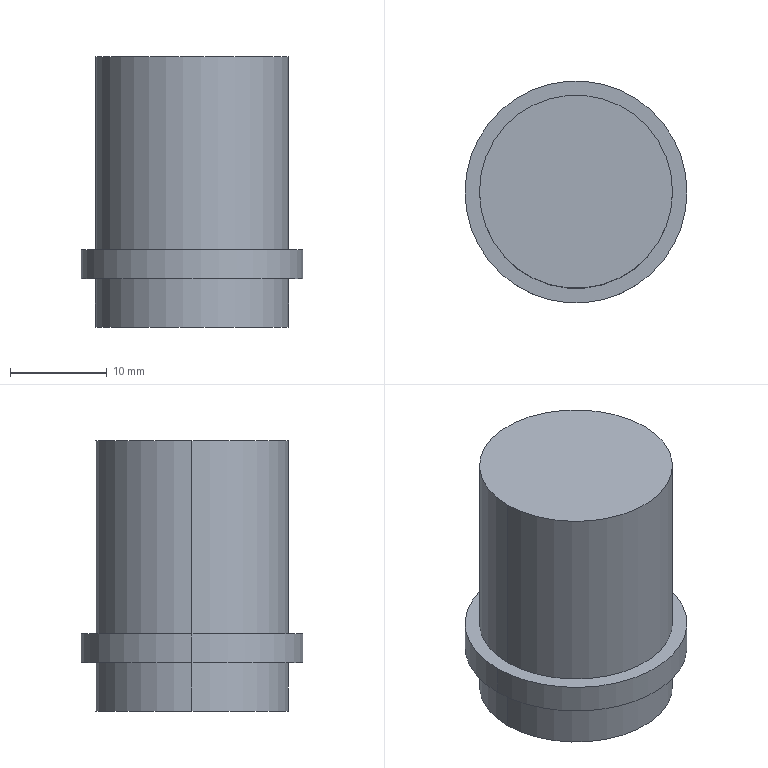Part | SolidWorks | features ICE 2, Extrusion 1 | 1 solid | 10 faces | box 23 x 23 x 28 mm | volume 9100 mm3 | cylinder 6 | plane 4 | commonest cylinder face diameters 20 x4 23 x2
STEP:
#1=CARTESIAN_POINT('',(10.,0.,28.));
#2=VERTEX_POINT('',#1);
#3=CARTESIAN_POINT('',(-10.,0.,28.));
#4=VERTEX_POINT('',#3);
#5=CARTESIAN_POINT('',(0.,0.,28.));
#6=DIRECTION('',(0.,0.,1.));
#7=DIRECTION('',(1.,0.,0.));
#8=AXIS2_PLACEMENT_3D('',#5,#6,#7);
#9=CIRCLE('',#8,10.);
#10=EDGE_CURVE('',#2,#4,#9,.T.);
#11=ORIENTED_EDGE('',*,*,#10,.F.);
#12=CARTESIAN_POINT('',(10.,0.,8.));
#13=VERTEX_POINT('',#12);
#14=CARTESIAN_POINT('',(10.,0.,28.));
#15=DIRECTION('',(0.,0.,-1.));
#16=VECTOR('',#15,1000.);
#17=LINE('',#14,#16);
#18=EDGE_CURVE('',#2,#13,#17,.T.);
#19=ORIENTED_EDGE('',*,*,#18,.T.);
#20=CARTESIAN_POINT('',(-10.,0.,8.));
#21=VERTEX_POINT('',#20);
#22=CARTESIAN_POINT('',(0.,0.,8.));
#23=DIRECTION('',(0.,0.,1.));
#24=DIRECTION('',(1.,0.,0.));
#25=AXIS2_PLACEMENT_3D('',#22,#23,#24);
#26=CIRCLE('',#25,10.);
#27=EDGE_CURVE('',#13,#21,#26,.T.);
#28=ORIENTED_EDGE('',*,*,#27,.T.);
#29=CARTESIAN_POINT('',(-10.,0.,28.));
#30=DIRECTION('',(0.,0.,-1.));
#31=VECTOR('',#30,1000.);
#32=LINE('',#29,#31);
#33=EDGE_CURVE('',#4,#21,#32,.T.);
#34=ORIENTED_EDGE('',*,*,#33,.F.);
#35=EDGE_LOOP('',(#11,#19,#28,#34));
#36=FACE_OUTER_BOUND('',#35,.T.);
#37=CARTESIAN_POINT('',(0.,0.,28.));
#38=DIRECTION('',(0.,0.,-1.));
#39=DIRECTION('',(-1.,0.,0.));
#40=AXIS2_PLACEMENT_3D('',#37,#38,#39);
#41=CYLINDRICAL_SURFACE('',#40,10.);
#42=ADVANCED_FACE('',(#36),#41,.T.);
#43=CARTESIAN_POINT('',(11.5,0.,8.));
#44=VERTEX_POINT('',#43);
#45=CARTESIAN_POINT('',(-11.5,0.,8.));
#46=VERTEX_POINT('',#45);
#47=CARTESIAN_POINT('',(0.,0.,8.));
#48=DIRECTION('',(0.,0.,1.));
#49=DIRECTION('',(1.,0.,0.));
#50=AXIS2_PLACEMENT_3D('',#47,#48,#49);
#51=CIRCLE('',#50,11.5);
#52=EDGE_CURVE('',#44,#46,#51,.T.);
#53=ORIENTED_EDGE('',*,*,#52,.F.);
#54=CARTESIAN_POINT('',(11.5,0.,5.));
#55=VERTEX_POINT('',#54);
#56=CARTESIAN_POINT('',(11.5,0.,8.));
#57=DIRECTION('',(0.,0.,-1.));
#58=VECTOR('',#57,1000.);
#59=LINE('',#56,#58);
#60=EDGE_CURVE('',#44,#55,#59,.T.);
#61=ORIENTED_EDGE('',*,*,#60,.T.);
#62=CARTESIAN_POINT('',(-11.5,0.,5.));
#63=VERTEX_POINT('',#62);
#64=CARTESIAN_POINT('',(0.,0.,5.));
#65=DIRECTION('',(0.,0.,1.));
#66=DIRECTION('',(1.,0.,0.));
#67=AXIS2_PLACEMENT_3D('',#64,#65,#66);
#68=CIRCLE('',#67,11.5);
#69=EDGE_CURVE('',#55,#63,#68,.T.);
#70=ORIENTED_EDGE('',*,*,#69,.T.);
#71=CARTESIAN_POINT('',(-11.5,0.,8.));
#72=DIRECTION('',(0.,0.,-1.));
#73=VECTOR('',#72,1000.);
#74=LINE('',#71,#73);
#75=EDGE_CURVE('',#46,#63,#74,.T.);
#76=ORIENTED_EDGE('',*,*,#75,.F.);
#77=EDGE_LOOP('',(#53,#61,#70,#76));
#78=FACE_OUTER_BOUND('',#77,.T.);
#79=CARTESIAN_POINT('',(0.,0.,8.));
#80=DIRECTION('',(0.,0.,-1.));
#81=DIRECTION('',(-1.,0.,0.));
#82=AXIS2_PLACEMENT_3D('',#79,#80,#81);
#83=CYLINDRICAL_SURFACE('',#82,11.5);
#84=ADVANCED_FACE('',(#78),#83,.T.);
#85=CARTESIAN_POINT('',(10.,0.,5.));
#86=VERTEX_POINT('',#85);
#87=CARTESIAN_POINT('',(-10.,0.,5.));
#88=VERTEX_POINT('',#87);
#89=CARTESIAN_POINT('',(0.,0.,5.));
#90=DIRECTION('',(0.,0.,1.));
#91=DIRECTION('',(1.,0.,0.));
#92=AXIS2_PLACEMENT_3D('',#89,#90,#91);
#93=CIRCLE('',#92,10.);
#94=EDGE_CURVE('',#86,#88,#93,.T.);
#95=ORIENTED_EDGE('',*,*,#94,.F.);
#96=CARTESIAN_POINT('',(10.,0.,0.));
#97=VERTEX_POINT('',#96);
#98=CARTESIAN_POINT('',(10.,0.,5.));
#99=DIRECTION('',(0.,0.,-1.));
#100=VECTOR('',#99,1000.);
#101=LINE('',#98,#100);
#102=EDGE_CURVE('',#86,#97,#101,.T.);
#103=ORIENTED_EDGE('',*,*,#102,.T.);
#104=CARTESIAN_POINT('',(-10.,0.,0.));
#105=VERTEX_POINT('',#104);
#106=CARTESIAN_POINT('',(0.,0.,0.));
#107=DIRECTION('',(0.,0.,1.));
#108=DIRECTION('',(1.,0.,0.));
#109=AXIS2_PLACEMENT_3D('',#106,#107,#108);
#110=CIRCLE('',#109,10.);
#111=EDGE_CURVE('',#97,#105,#110,.T.);
#112=ORIENTED_EDGE('',*,*,#111,.T.);
#113=CARTESIAN_POINT('',(-10.,0.,5.));
#114=DIRECTION('',(0.,0.,-1.));
#115=VECTOR('',#114,1000.);
#116=LINE('',#113,#115);
#117=EDGE_CURVE('',#88,#105,#116,.T.);
#118=ORIENTED_EDGE('',*,*,#117,.F.);
#119=EDGE_LOOP('',(#95,#103,#112,#118));
#120=FACE_OUTER_BOUND('',#119,.T.);
#121=CARTESIAN_POINT('',(0.,0.,5.));
#122=DIRECTION('',(0.,0.,-1.));
#123=DIRECTION('',(-1.,0.,0.));
#124=AXIS2_PLACEMENT_3D('',#121,#122,#123);
#125=CYLINDRICAL_SURFACE('',#124,10.);
#126=ADVANCED_FACE('',(#120),#125,.T.);
#127=ORIENTED_EDGE('',*,*,#102,.F.);
#128=CARTESIAN_POINT('',(0.,0.,5.));
#129=DIRECTION('',(0.,0.,1.));
#130=DIRECTION('',(1.,0.,0.));
#131=AXIS2_PLACEMENT_3D('',#128,#129,#130);
#132=CIRCLE('',#131,10.);
#133=EDGE_CURVE('',#88,#86,#132,.T.);
#134=ORIENTED_EDGE('',*,*,#133,.F.);
#135=ORIENTED_EDGE('',*,*,#117,.T.);
#136=CARTESIAN_POINT('',(0.,0.,0.));
#137=DIRECTION('',(0.,0.,1.));
#138=DIRECTION('',(1.,0.,0.));
#139=AXIS2_PLACEMENT_3D('',#136,#137,#138);
#140=CIRCLE('',#139,10.);
#141=EDGE_CURVE('',#105,#97,#140,.T.);
#142=ORIENTED_EDGE('',*,*,#141,.T.);
#143=EDGE_LOOP('',(#127,#134,#135,#142));
#144=FACE_OUTER_BOUND('',#143,.T.);
#145=CARTESIAN_POINT('',(0.,0.,5.));
#146=DIRECTION('',(0.,0.,-1.));
#147=DIRECTION('',(-1.,0.,0.));
#148=AXIS2_PLACEMENT_3D('',#145,#146,#147);
#149=CYLINDRICAL_SURFACE('',#148,10.);
#150=ADVANCED_FACE('',(#144),#149,.T.);
#151=ORIENTED_EDGE('',*,*,#141,.F.);
#152=ORIENTED_EDGE('',*,*,#111,.F.);
#153=EDGE_LOOP('',(#151,#152));
#154=FACE_OUTER_BOUND('',#153,.T.);
#155=CARTESIAN_POINT('',(0.,0.,0.));
#156=DIRECTION('',(0.,0.,1.));
#157=DIRECTION('',(1.,0.,0.));
#158=AXIS2_PLACEMENT_3D('',#155,#156,#157);
#159=PLANE('',#158);
#160=ADVANCED_FACE('',(#154),#159,.F.);
#161=ORIENTED_EDGE('',*,*,#60,.F.);
#162=CARTESIAN_POINT('',(0.,0.,8.));
#163=DIRECTION('',(0.,0.,1.));
#164=DIRECTION('',(1.,0.,0.));
#165=AXIS2_PLACEMENT_3D('',#162,#163,#164);
#166=CIRCLE('',#165,11.5);
#167=EDGE_CURVE('',#46,#44,#166,.T.);
#168=ORIENTED_EDGE('',*,*,#167,.F.);
#169=ORIENTED_EDGE('',*,*,#75,.T.);
#170=CARTESIAN_POINT('',(0.,0.,5.));
#171=DIRECTION('',(0.,0.,1.));
#172=DIRECTION('',(1.,0.,0.));
#173=AXIS2_PLACEMENT_3D('',#170,#171,#172);
#174=CIRCLE('',#173,11.5);
#175=EDGE_CURVE('',#63,#55,#174,.T.);
#176=ORIENTED_EDGE('',*,*,#175,.T.);
#177=EDGE_LOOP('',(#161,#168,#169,#176));
#178=FACE_OUTER_BOUND('',#177,.T.);
#179=CARTESIAN_POINT('',(0.,0.,8.));
#180=DIRECTION('',(0.,0.,-1.));
#181=DIRECTION('',(-1.,0.,0.));
#182=AXIS2_PLACEMENT_3D('',#179,#180,#181);
#183=CYLINDRICAL_SURFACE('',#182,11.5);
#184=ADVANCED_FACE('',(#178),#183,.T.);
#185=CARTESIAN_POINT('',(0.,0.,8.));
#186=DIRECTION('',(0.,0.,1.));
#187=DIRECTION('',(1.,0.,0.));
#188=AXIS2_PLACEMENT_3D('',#185,#186,#187);
#189=CIRCLE('',#188,10.);
#190=EDGE_CURVE('',#21,#13,#189,.T.);
#191=ORIENTED_EDGE('',*,*,#190,.F.);
#192=ORIENTED_EDGE('',*,*,#27,.F.);
#193=EDGE_LOOP('',(#191,#192));
#194=FACE_BOUND('',#193,.T.);
#195=ORIENTED_EDGE('',*,*,#167,.T.);
#196=ORIENTED_EDGE('',*,*,#52,.T.);
#197=EDGE_LOOP('',(#195,#196));
#198=FACE_OUTER_BOUND('',#197,.T.);
#199=CARTESIAN_POINT('',(0.,0.,8.));
#200=DIRECTION('',(0.,0.,1.));
#201=DIRECTION('',(1.,0.,0.));
#202=AXIS2_PLACEMENT_3D('',#199,#200,#201);
#203=PLANE('',#202);
#204=ADVANCED_FACE('',(#194,#198),#203,.T.);
#205=ORIENTED_EDGE('',*,*,#133,.T.);
#206=ORIENTED_EDGE('',*,*,#94,.T.);
#207=EDGE_LOOP('',(#205,#206));
#208=FACE_BOUND('',#207,.T.);
#209=ORIENTED_EDGE('',*,*,#175,.F.);
#210=ORIENTED_EDGE('',*,*,#69,.F.);
#211=EDGE_LOOP('',(#209,#210));
#212=FACE_OUTER_BOUND('',#211,.T.);
#213=CARTESIAN_POINT('',(0.,0.,5.));
#214=DIRECTION('',(0.,0.,1.));
#215=DIRECTION('',(1.,0.,0.));
#216=AXIS2_PLACEMENT_3D('',#213,#214,#215);
#217=PLANE('',#216);
#218=ADVANCED_FACE('',(#208,#212),#217,.F.);
#219=ORIENTED_EDGE('',*,*,#18,.F.);
#220=CARTESIAN_POINT('',(0.,0.,28.));
#221=DIRECTION('',(0.,0.,1.));
#222=DIRECTION('',(1.,0.,0.));
#223=AXIS2_PLACEMENT_3D('',#220,#221,#222);
#224=CIRCLE('',#223,10.);
#225=EDGE_CURVE('',#4,#2,#224,.T.);
#226=ORIENTED_EDGE('',*,*,#225,.F.);
#227=ORIENTED_EDGE('',*,*,#33,.T.);
#228=ORIENTED_EDGE('',*,*,#190,.T.);
#229=EDGE_LOOP('',(#219,#226,#227,#228));
#230=FACE_OUTER_BOUND('',#229,.T.);
#231=CARTESIAN_POINT('',(0.,0.,28.));
#232=DIRECTION('',(0.,0.,-1.));
#233=DIRECTION('',(-1.,0.,0.));
#234=AXIS2_PLACEMENT_3D('',#231,#232,#233);
#235=CYLINDRICAL_SURFACE('',#234,10.);
#236=ADVANCED_FACE('',(#230),#235,.T.);
#237=ORIENTED_EDGE('',*,*,#225,.T.);
#238=ORIENTED_EDGE('',*,*,#10,.T.);
#239=EDGE_LOOP('',(#237,#238));
#240=FACE_OUTER_BOUND('',#239,.T.);
#241=CARTESIAN_POINT('',(0.,0.,28.));
#242=DIRECTION('',(0.,0.,1.));
#243=DIRECTION('',(1.,0.,0.));
#244=AXIS2_PLACEMENT_3D('',#241,#242,#243);
#245=PLANE('',#244);
#246=ADVANCED_FACE('',(#240),#245,.T.);
#247=CLOSED_SHELL('',(#42,#84,#126,#150,#160,#184,#204,#218,#236,#246));
#248=MANIFOLD_SOLID_BREP('',#247);
#249=CARTESIAN_POINT('',(0.,0.,0.));
#250=DIRECTION('',(0.,0.,1.));
#251=DIRECTION('',(1.,0.,0.));
#252=AXIS2_PLACEMENT_3D('',#249,#250,#251);
#253=(LENGTH_UNIT()NAMED_UNIT(*)SI_UNIT(.MILLI.,.METRE.));
#254=UNCERTAINTY_MEASURE_WITH_UNIT(LENGTH_MEASURE(0.00001),#253,'','');
#255=(NAMED_UNIT(*)PLANE_ANGLE_UNIT()SI_UNIT($,.RADIAN.));
#256=(NAMED_UNIT(*)SI_UNIT($,.STERADIAN.)SOLID_ANGLE_UNIT());
#257=(GEOMETRIC_REPRESENTATION_CONTEXT(3)GLOBAL_UNCERTAINTY_ASSIGNED_CONTEXT((#254))GLOBAL_UNIT_ASSIGNED_CONTEXT((#253,#255,#256))REPRESENTATION_CONTEXT('',''));
#258=ADVANCED_BREP_SHAPE_REPRESENTATION('',(#248,#252),#257);